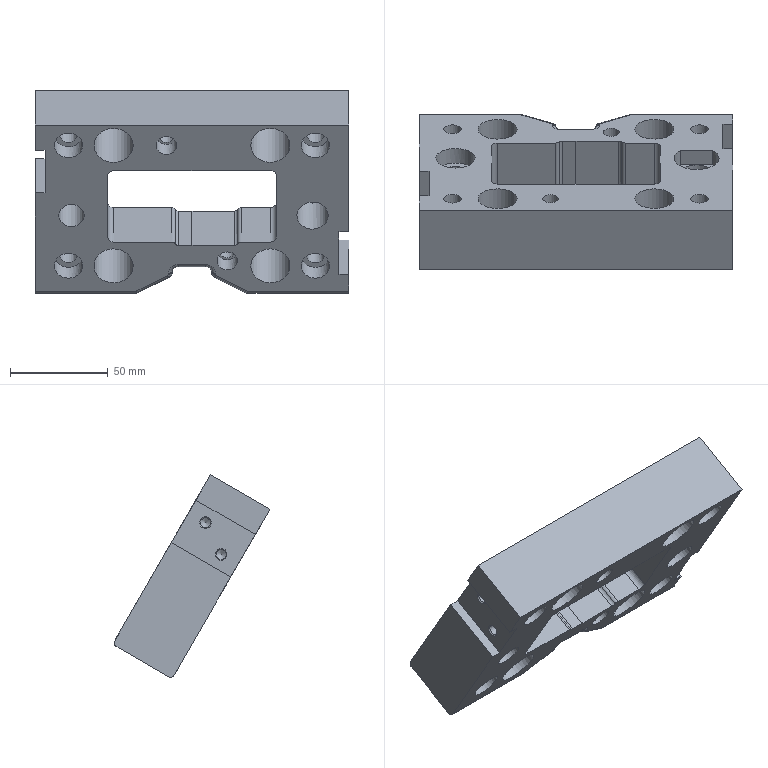Part | NX | features solid 2 | 1 solid | 104 faces | box 160 x 79.58 x 103.37 mm | volume 327345 mm3 | cylinder 42 | plane 38 | spline 8 | torus 8 | cone 8 | commonest cylinder face diameters 4 x14 20 x5 5 x4 6 x4 9.007 x4 14.508 x4